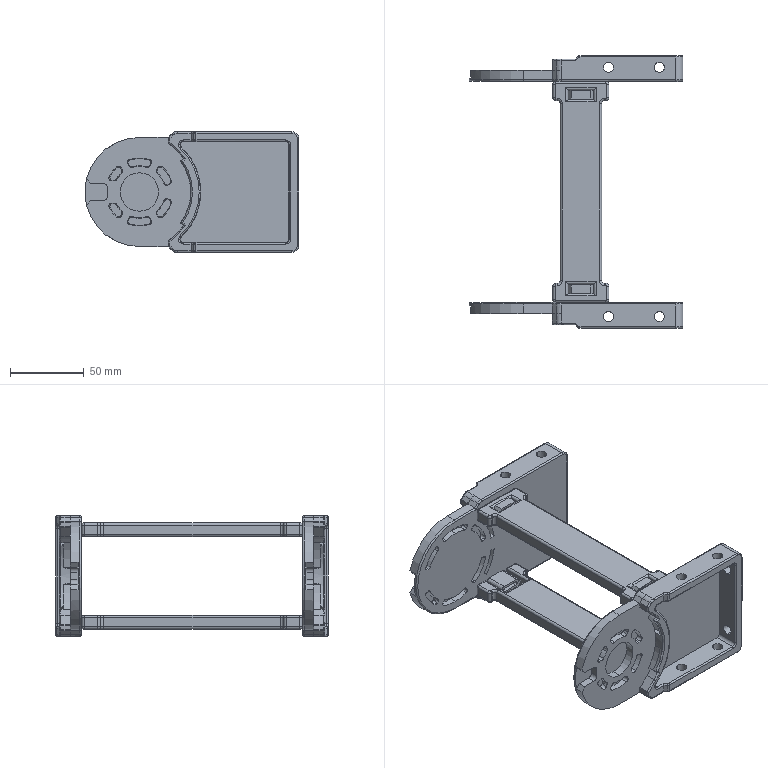Part | SolidWorks | features MirrorCompFeat 1, ReferencePattern 1 | 4 solids | 878 faces | box 145.118 x 185 x 82 mm | volume 205797 mm3 | cylinder 366 | plane 288 | cone 114 | torus 88 | spline 14 | sphere 8 | commonest cylinder face diameters 4 x92 3 x80 3.2 x72 2 x66 7 x24 4.4 x12